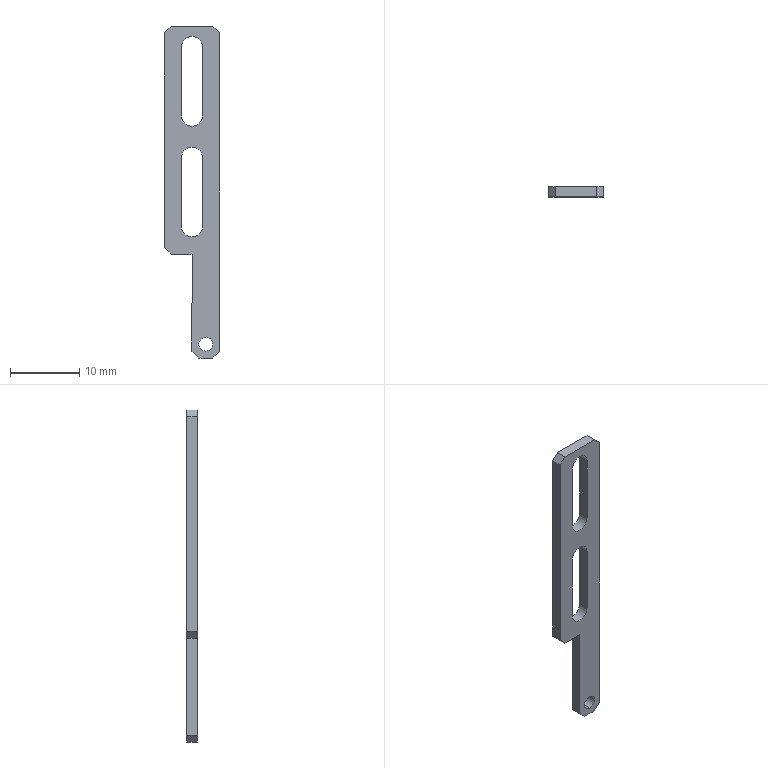Part | SolidWorks | features ICE 3, Chamfer 1, Extrusion 1, HoleWzd 1 | 1 solid | 25 faces | box 8 x 1.5 x 48 mm | volume 366.332 mm3 | plane 17 | cylinder 8 | commonest cylinder face diameters 3 x6 2 x2
STEP:
#1=CARTESIAN_POINT('',(5.5,0.,-3.));
#2=VERTEX_POINT('',#1);
#3=CARTESIAN_POINT('',(4.,0.,-1.5));
#4=VERTEX_POINT('',#3);
#5=CARTESIAN_POINT('',(4.,0.,-3.));
#6=DIRECTION('',(0.,-1.,0.));
#7=DIRECTION('',(0.,0.,-1.));
#8=AXIS2_PLACEMENT_3D('',#5,#6,#7);
#9=CIRCLE('',#8,1.5);
#10=EDGE_CURVE('',#2,#4,#9,.T.);
#11=ORIENTED_EDGE('',*,*,#10,.T.);
#12=CARTESIAN_POINT('',(4.,1.5,-1.5));
#13=VERTEX_POINT('',#12);
#14=CARTESIAN_POINT('',(4.,-8.5,-1.5));
#15=DIRECTION('',(0.,1.,0.));
#16=VECTOR('',#15,1000.);
#17=LINE('',#14,#16);
#18=EDGE_CURVE('',#4,#13,#17,.T.);
#19=ORIENTED_EDGE('',*,*,#18,.T.);
#20=CARTESIAN_POINT('',(5.5,1.5,-3.));
#21=VERTEX_POINT('',#20);
#22=CARTESIAN_POINT('',(4.,1.5,-3.));
#23=DIRECTION('',(0.,1.,0.));
#24=DIRECTION('',(0.,0.,1.));
#25=AXIS2_PLACEMENT_3D('',#22,#23,#24);
#26=CIRCLE('',#25,1.5);
#27=EDGE_CURVE('',#13,#21,#26,.T.);
#28=ORIENTED_EDGE('',*,*,#27,.T.);
#29=CARTESIAN_POINT('',(5.5,-8.5,-3.));
#30=DIRECTION('',(0.,1.,0.));
#31=VECTOR('',#30,1000.);
#32=LINE('',#29,#31);
#33=EDGE_CURVE('',#2,#21,#32,.T.);
#34=ORIENTED_EDGE('',*,*,#33,.F.);
#35=EDGE_LOOP('',(#11,#19,#28,#34));
#36=FACE_OUTER_BOUND('',#35,.T.);
#37=CARTESIAN_POINT('',(4.,-8.5,-3.));
#38=DIRECTION('',(0.,1.,0.));
#39=DIRECTION('',(0.,0.,1.));
#40=AXIS2_PLACEMENT_3D('',#37,#38,#39);
#41=CYLINDRICAL_SURFACE('',#40,1.5);
#42=ADVANCED_FACE('',(#36),#41,.F.);
#43=CARTESIAN_POINT('',(5.5,0.,-19.));
#44=VERTEX_POINT('',#43);
#45=CARTESIAN_POINT('',(4.,0.,-17.5));
#46=VERTEX_POINT('',#45);
#47=CARTESIAN_POINT('',(4.,0.,-19.));
#48=DIRECTION('',(0.,-1.,0.));
#49=DIRECTION('',(0.,0.,-1.));
#50=AXIS2_PLACEMENT_3D('',#47,#48,#49);
#51=CIRCLE('',#50,1.5);
#52=EDGE_CURVE('',#44,#46,#51,.T.);
#53=ORIENTED_EDGE('',*,*,#52,.T.);
#54=CARTESIAN_POINT('',(4.,1.5,-17.5));
#55=VERTEX_POINT('',#54);
#56=CARTESIAN_POINT('',(4.,-8.5,-17.5));
#57=DIRECTION('',(0.,1.,0.));
#58=VECTOR('',#57,1000.);
#59=LINE('',#56,#58);
#60=EDGE_CURVE('',#46,#55,#59,.T.);
#61=ORIENTED_EDGE('',*,*,#60,.T.);
#62=CARTESIAN_POINT('',(5.5,1.5,-19.));
#63=VERTEX_POINT('',#62);
#64=CARTESIAN_POINT('',(4.,1.5,-19.));
#65=DIRECTION('',(0.,1.,0.));
#66=DIRECTION('',(0.,0.,1.));
#67=AXIS2_PLACEMENT_3D('',#64,#65,#66);
#68=CIRCLE('',#67,1.5);
#69=EDGE_CURVE('',#55,#63,#68,.T.);
#70=ORIENTED_EDGE('',*,*,#69,.T.);
#71=CARTESIAN_POINT('',(5.5,-8.5,-19.));
#72=DIRECTION('',(0.,1.,0.));
#73=VECTOR('',#72,1000.);
#74=LINE('',#71,#73);
#75=EDGE_CURVE('',#44,#63,#74,.T.);
#76=ORIENTED_EDGE('',*,*,#75,.F.);
#77=EDGE_LOOP('',(#53,#61,#70,#76));
#78=FACE_OUTER_BOUND('',#77,.T.);
#79=CARTESIAN_POINT('',(4.,-8.5,-19.));
#80=DIRECTION('',(0.,1.,0.));
#81=DIRECTION('',(0.,0.,1.));
#82=AXIS2_PLACEMENT_3D('',#79,#80,#81);
#83=CYLINDRICAL_SURFACE('',#82,1.5);
#84=ADVANCED_FACE('',(#78),#83,.F.);
#85=CARTESIAN_POINT('',(6.,0.,-45.));
#86=VERTEX_POINT('',#85);
#87=CARTESIAN_POINT('',(6.,0.,-47.));
#88=VERTEX_POINT('',#87);
#89=CARTESIAN_POINT('',(6.,0.,-46.));
#90=DIRECTION('',(0.,-1.,0.));
#91=DIRECTION('',(0.,0.,-1.));
#92=AXIS2_PLACEMENT_3D('',#89,#90,#91);
#93=CIRCLE('',#92,1.);
#94=EDGE_CURVE('',#86,#88,#93,.T.);
#95=ORIENTED_EDGE('',*,*,#94,.T.);
#96=CARTESIAN_POINT('',(6.,1.5,-47.));
#97=VERTEX_POINT('',#96);
#98=CARTESIAN_POINT('',(6.,1.5,-47.));
#99=DIRECTION('',(0.,1.,0.));
#100=VECTOR('',#99,1000.);
#101=LINE('',#98,#100);
#102=EDGE_CURVE('',#88,#97,#101,.T.);
#103=ORIENTED_EDGE('',*,*,#102,.T.);
#104=CARTESIAN_POINT('',(6.,1.5,-45.));
#105=VERTEX_POINT('',#104);
#106=CARTESIAN_POINT('',(6.,1.5,-46.));
#107=DIRECTION('',(0.,1.,0.));
#108=DIRECTION('',(0.,0.,1.));
#109=AXIS2_PLACEMENT_3D('',#106,#107,#108);
#110=CIRCLE('',#109,1.);
#111=EDGE_CURVE('',#97,#105,#110,.T.);
#112=ORIENTED_EDGE('',*,*,#111,.T.);
#113=CARTESIAN_POINT('',(6.,1.5,-45.));
#114=DIRECTION('',(0.,1.,0.));
#115=VECTOR('',#114,1000.);
#116=LINE('',#113,#115);
#117=EDGE_CURVE('',#86,#105,#116,.T.);
#118=ORIENTED_EDGE('',*,*,#117,.F.);
#119=EDGE_LOOP('',(#95,#103,#112,#118));
#120=FACE_OUTER_BOUND('',#119,.T.);
#121=CARTESIAN_POINT('',(6.,1.5,-46.));
#122=DIRECTION('',(0.,1.,0.));
#123=DIRECTION('',(0.,0.,1.));
#124=AXIS2_PLACEMENT_3D('',#121,#122,#123);
#125=CYLINDRICAL_SURFACE('',#124,1.);
#126=ADVANCED_FACE('',(#120),#125,.F.);
#127=CARTESIAN_POINT('',(0.,0.,-32.));
#128=VERTEX_POINT('',#127);
#129=CARTESIAN_POINT('',(0.,0.,-1.));
#130=VERTEX_POINT('',#129);
#131=CARTESIAN_POINT('',(0.,0.,0.));
#132=DIRECTION('',(0.,0.,1.));
#133=VECTOR('',#132,1000.);
#134=LINE('',#131,#133);
#135=EDGE_CURVE('',#128,#130,#134,.T.);
#136=ORIENTED_EDGE('',*,*,#135,.T.);
#137=CARTESIAN_POINT('',(0.,1.5,-1.));
#138=VERTEX_POINT('',#137);
#139=CARTESIAN_POINT('',(0.,1.5,-1.));
#140=DIRECTION('',(0.,1.,0.));
#141=VECTOR('',#140,1000.);
#142=LINE('',#139,#141);
#143=EDGE_CURVE('',#130,#138,#142,.T.);
#144=ORIENTED_EDGE('',*,*,#143,.T.);
#145=CARTESIAN_POINT('',(0.,1.5,-32.));
#146=VERTEX_POINT('',#145);
#147=CARTESIAN_POINT('',(0.,1.5,0.));
#148=DIRECTION('',(0.,0.,1.));
#149=VECTOR('',#148,1000.);
#150=LINE('',#147,#149);
#151=EDGE_CURVE('',#146,#138,#150,.T.);
#152=ORIENTED_EDGE('',*,*,#151,.F.);
#153=CARTESIAN_POINT('',(0.,1.5,-32.));
#154=DIRECTION('',(0.,-1.,0.));
#155=VECTOR('',#154,1000.);
#156=LINE('',#153,#155);
#157=EDGE_CURVE('',#146,#128,#156,.T.);
#158=ORIENTED_EDGE('',*,*,#157,.T.);
#159=EDGE_LOOP('',(#136,#144,#152,#158));
#160=FACE_OUTER_BOUND('',#159,.T.);
#161=CARTESIAN_POINT('',(0.,1.5,0.));
#162=DIRECTION('',(1.,0.,0.));
#163=DIRECTION('',(0.,0.,-1.));
#164=AXIS2_PLACEMENT_3D('',#161,#162,#163);
#165=PLANE('',#164);
#166=ADVANCED_FACE('',(#160),#165,.F.);
#167=CARTESIAN_POINT('',(1.,0.,0.));
#168=VERTEX_POINT('',#167);
#169=CARTESIAN_POINT('',(7.,0.,0.));
#170=VERTEX_POINT('',#169);
#171=CARTESIAN_POINT('',(0.,0.,0.));
#172=DIRECTION('',(1.,0.,0.));
#173=VECTOR('',#172,1000.);
#174=LINE('',#171,#173);
#175=EDGE_CURVE('',#168,#170,#174,.T.);
#176=ORIENTED_EDGE('',*,*,#175,.T.);
#177=CARTESIAN_POINT('',(7.,1.5,0.));
#178=VERTEX_POINT('',#177);
#179=CARTESIAN_POINT('',(7.,1.5,0.));
#180=DIRECTION('',(0.,1.,0.));
#181=VECTOR('',#180,1000.);
#182=LINE('',#179,#181);
#183=EDGE_CURVE('',#170,#178,#182,.T.);
#184=ORIENTED_EDGE('',*,*,#183,.T.);
#185=CARTESIAN_POINT('',(1.,1.5,0.));
#186=VERTEX_POINT('',#185);
#187=CARTESIAN_POINT('',(0.,1.5,0.));
#188=DIRECTION('',(1.,0.,0.));
#189=VECTOR('',#188,1000.);
#190=LINE('',#187,#189);
#191=EDGE_CURVE('',#186,#178,#190,.T.);
#192=ORIENTED_EDGE('',*,*,#191,.F.);
#193=CARTESIAN_POINT('',(1.,1.5,0.));
#194=DIRECTION('',(0.,-1.,0.));
#195=VECTOR('',#194,1000.);
#196=LINE('',#193,#195);
#197=EDGE_CURVE('',#186,#168,#196,.T.);
#198=ORIENTED_EDGE('',*,*,#197,.T.);
#199=EDGE_LOOP('',(#176,#184,#192,#198));
#200=FACE_OUTER_BOUND('',#199,.T.);
#201=CARTESIAN_POINT('',(0.,1.5,0.));
#202=DIRECTION('',(0.,0.,-1.));
#203=DIRECTION('',(-1.,0.,0.));
#204=AXIS2_PLACEMENT_3D('',#201,#202,#203);
#205=PLANE('',#204);
#206=ADVANCED_FACE('',(#200),#205,.F.);
#207=CARTESIAN_POINT('',(8.,1.5,-1.));
#208=VERTEX_POINT('',#207);
#209=CARTESIAN_POINT('',(8.,1.5,-47.));
#210=VERTEX_POINT('',#209);
#211=CARTESIAN_POINT('',(8.,1.5,0.));
#212=DIRECTION('',(0.,0.,-1.));
#213=VECTOR('',#212,1000.);
#214=LINE('',#211,#213);
#215=EDGE_CURVE('',#208,#210,#214,.T.);
#216=ORIENTED_EDGE('',*,*,#215,.F.);
#217=CARTESIAN_POINT('',(8.,0.,-1.));
#218=VERTEX_POINT('',#217);
#219=CARTESIAN_POINT('',(8.,1.5,-1.));
#220=DIRECTION('',(0.,-1.,0.));
#221=VECTOR('',#220,1000.);
#222=LINE('',#219,#221);
#223=EDGE_CURVE('',#208,#218,#222,.T.);
#224=ORIENTED_EDGE('',*,*,#223,.T.);
#225=CARTESIAN_POINT('',(8.,0.,-47.));
#226=VERTEX_POINT('',#225);
#227=CARTESIAN_POINT('',(8.,0.,0.));
#228=DIRECTION('',(0.,0.,-1.));
#229=VECTOR('',#228,1000.);
#230=LINE('',#227,#229);
#231=EDGE_CURVE('',#218,#226,#230,.T.);
#232=ORIENTED_EDGE('',*,*,#231,.T.);
#233=CARTESIAN_POINT('',(8.,1.5,-47.));
#234=DIRECTION('',(0.,1.,0.));
#235=VECTOR('',#234,1000.);
#236=LINE('',#233,#235);
#237=EDGE_CURVE('',#226,#210,#236,.T.);
#238=ORIENTED_EDGE('',*,*,#237,.T.);
#239=EDGE_LOOP('',(#216,#224,#232,#238));
#240=FACE_OUTER_BOUND('',#239,.T.);
#241=CARTESIAN_POINT('',(8.,1.5,0.));
#242=DIRECTION('',(-1.,0.,0.));
#243=DIRECTION('',(0.,0.,1.));
#244=AXIS2_PLACEMENT_3D('',#241,#242,#243);
#245=PLANE('',#244);
#246=ADVANCED_FACE('',(#240),#245,.F.);
#247=CARTESIAN_POINT('',(7.,0.,-48.));
#248=VERTEX_POINT('',#247);
#249=CARTESIAN_POINT('',(5.,0.,-48.));
#250=VERTEX_POINT('',#249);
#251=CARTESIAN_POINT('',(0.,0.,-48.));
#252=DIRECTION('',(-1.,0.,0.));
#253=VECTOR('',#252,1000.);
#254=LINE('',#251,#253);
#255=EDGE_CURVE('',#248,#250,#254,.T.);
#256=ORIENTED_EDGE('',*,*,#255,.T.);
#257=CARTESIAN_POINT('',(5.,1.5,-48.));
#258=VERTEX_POINT('',#257);
#259=CARTESIAN_POINT('',(5.,1.5,-48.));
#260=DIRECTION('',(0.,1.,0.));
#261=VECTOR('',#260,1000.);
#262=LINE('',#259,#261);
#263=EDGE_CURVE('',#250,#258,#262,.T.);
#264=ORIENTED_EDGE('',*,*,#263,.T.);
#265=CARTESIAN_POINT('',(7.,1.5,-48.));
#266=VERTEX_POINT('',#265);
#267=CARTESIAN_POINT('',(0.,1.5,-48.));
#268=DIRECTION('',(-1.,0.,0.));
#269=VECTOR('',#268,1000.);
#270=LINE('',#267,#269);
#271=EDGE_CURVE('',#266,#258,#270,.T.);
#272=ORIENTED_EDGE('',*,*,#271,.F.);
#273=CARTESIAN_POINT('',(7.,1.5,-48.));
#274=DIRECTION('',(0.,-1.,0.));
#275=VECTOR('',#274,1000.);
#276=LINE('',#273,#275);
#277=EDGE_CURVE('',#266,#248,#276,.T.);
#278=ORIENTED_EDGE('',*,*,#277,.T.);
#279=EDGE_LOOP('',(#256,#264,#272,#278));
#280=FACE_OUTER_BOUND('',#279,.T.);
#281=CARTESIAN_POINT('',(0.,1.5,-48.));
#282=DIRECTION('',(0.,0.,1.));
#283=DIRECTION('',(1.,0.,0.));
#284=AXIS2_PLACEMENT_3D('',#281,#282,#283);
#285=PLANE('',#284);
#286=ADVANCED_FACE('',(#280),#285,.F.);
#287=CARTESIAN_POINT('',(5.5,1.5,-13.));
#288=VERTEX_POINT('',#287);
#289=CARTESIAN_POINT('',(5.5,1.5,-3.));
#290=DIRECTION('',(0.,0.,-1.));
#291=VECTOR('',#290,1000.);
#292=LINE('',#289,#291);
#293=EDGE_CURVE('',#21,#288,#292,.T.);
#294=ORIENTED_EDGE('',*,*,#293,.F.);
#295=ORIENTED_EDGE('',*,*,#27,.F.);
#296=CARTESIAN_POINT('',(2.5,1.5,-3.));
#297=VERTEX_POINT('',#296);
#298=CARTESIAN_POINT('',(4.,1.5,-3.));
#299=DIRECTION('',(0.,1.,0.));
#300=DIRECTION('',(0.,0.,1.));
#301=AXIS2_PLACEMENT_3D('',#298,#299,#300);
#302=CIRCLE('',#301,1.5);
#303=EDGE_CURVE('',#297,#13,#302,.T.);
#304=ORIENTED_EDGE('',*,*,#303,.F.);
#305=CARTESIAN_POINT('',(2.5,1.5,-13.));
#306=VERTEX_POINT('',#305);
#307=CARTESIAN_POINT('',(2.5,1.5,-3.));
#308=DIRECTION('',(0.,0.,1.));
#309=VECTOR('',#308,1000.);
#310=LINE('',#307,#309);
#311=EDGE_CURVE('',#306,#297,#310,.T.);
#312=ORIENTED_EDGE('',*,*,#311,.F.);
#313=CARTESIAN_POINT('',(4.,1.5,-13.));
#314=DIRECTION('',(0.,1.,0.));
#315=DIRECTION('',(0.,0.,1.));
#316=AXIS2_PLACEMENT_3D('',#313,#314,#315);
#317=CIRCLE('',#316,1.5);
#318=EDGE_CURVE('',#288,#306,#317,.T.);
#319=ORIENTED_EDGE('',*,*,#318,.F.);
#320=EDGE_LOOP('',(#294,#295,#304,#312,#319));
#321=FACE_BOUND('',#320,.T.);
#322=CARTESIAN_POINT('',(2.5,1.5,-29.));
#323=VERTEX_POINT('',#322);
#324=CARTESIAN_POINT('',(2.5,1.5,-19.));
#325=VERTEX_POINT('',#324);
#326=CARTESIAN_POINT('',(2.5,1.5,-29.));
#327=DIRECTION('',(0.,0.,1.));
#328=VECTOR('',#327,1000.);
#329=LINE('',#326,#328);
#330=EDGE_CURVE('',#323,#325,#329,.T.);
#331=ORIENTED_EDGE('',*,*,#330,.F.);
#332=CARTESIAN_POINT('',(5.5,1.5,-29.));
#333=VERTEX_POINT('',#332);
#334=CARTESIAN_POINT('',(4.,1.5,-29.));
#335=DIRECTION('',(0.,1.,0.));
#336=DIRECTION('',(0.,0.,1.));
#337=AXIS2_PLACEMENT_3D('',#334,#335,#336);
#338=CIRCLE('',#337,1.5);
#339=EDGE_CURVE('',#333,#323,#338,.T.);
#340=ORIENTED_EDGE('',*,*,#339,.F.);
#341=CARTESIAN_POINT('',(5.5,1.5,-29.));
#342=DIRECTION('',(0.,0.,-1.));
#343=VECTOR('',#342,1000.);
#344=LINE('',#341,#343);
#345=EDGE_CURVE('',#63,#333,#344,.T.);
#346=ORIENTED_EDGE('',*,*,#345,.F.);
#347=ORIENTED_EDGE('',*,*,#69,.F.);
#348=CARTESIAN_POINT('',(4.,1.5,-19.));
#349=DIRECTION('',(0.,1.,0.));
#350=DIRECTION('',(0.,0.,1.));
#351=AXIS2_PLACEMENT_3D('',#348,#349,#350);
#352=CIRCLE('',#351,1.5);
#353=EDGE_CURVE('',#325,#55,#352,.T.);
#354=ORIENTED_EDGE('',*,*,#353,.F.);
#355=EDGE_LOOP('',(#331,#340,#346,#347,#354));
#356=FACE_BOUND('',#355,.T.);
#357=CARTESIAN_POINT('',(6.,1.5,-46.));
#358=DIRECTION('',(0.,1.,0.));
#359=DIRECTION('',(0.,0.,1.));
#360=AXIS2_PLACEMENT_3D('',#357,#358,#359);
#361=CIRCLE('',#360,1.);
#362=EDGE_CURVE('',#105,#97,#361,.T.);
#363=ORIENTED_EDGE('',*,*,#362,.F.);
#364=ORIENTED_EDGE('',*,*,#111,.F.);
#365=EDGE_LOOP('',(#363,#364));
#366=FACE_BOUND('',#365,.T.);
#367=ORIENTED_EDGE('',*,*,#191,.T.);
#368=CARTESIAN_POINT('',(8.,1.5,-1.));
#369=DIRECTION('',(0.7071,0.,-0.7071));
#370=VECTOR('',#369,1000.);
#371=LINE('',#368,#370);
#372=EDGE_CURVE('',#178,#208,#371,.T.);
#373=ORIENTED_EDGE('',*,*,#372,.T.);
#374=ORIENTED_EDGE('',*,*,#215,.T.);
#375=CARTESIAN_POINT('',(7.,1.5,-48.));
#376=DIRECTION('',(-0.7071,0.,-0.7071));
#377=VECTOR('',#376,1000.);
#378=LINE('',#375,#377);
#379=EDGE_CURVE('',#210,#266,#378,.T.);
#380=ORIENTED_EDGE('',*,*,#379,.T.);
#381=ORIENTED_EDGE('',*,*,#271,.T.);
#382=CARTESIAN_POINT('',(4.,1.5,-47.));
#383=VERTEX_POINT('',#382);
#384=CARTESIAN_POINT('',(5.,1.5,-48.));
#385=DIRECTION('',(-0.7071,0.,0.7071));
#386=VECTOR('',#385,1000.);
#387=LINE('',#384,#386);
#388=EDGE_CURVE('',#258,#383,#387,.T.);
#389=ORIENTED_EDGE('',*,*,#388,.T.);
#390=CARTESIAN_POINT('',(4.,1.5,-33.));
#391=VERTEX_POINT('',#390);
#392=CARTESIAN_POINT('',(4.,1.5,-48.));
#393=DIRECTION('',(0.,0.,-1.));
#394=VECTOR('',#393,1000.);
#395=LINE('',#392,#394);
#396=EDGE_CURVE('',#391,#383,#395,.T.);
#397=ORIENTED_EDGE('',*,*,#396,.F.);
#398=CARTESIAN_POINT('',(1.,1.5,-33.));
#399=VERTEX_POINT('',#398);
#400=CARTESIAN_POINT('',(0.,1.5,-33.));
#401=DIRECTION('',(1.,0.,0.));
#402=VECTOR('',#401,1000.);
#403=LINE('',#400,#402);
#404=EDGE_CURVE('',#399,#391,#403,.T.);
#405=ORIENTED_EDGE('',*,*,#404,.F.);
#406=CARTESIAN_POINT('',(1.,1.5,-33.));
#407=DIRECTION('',(-0.7071,0.,0.7071));
#408=VECTOR('',#407,1000.);
#409=LINE('',#406,#408);
#410=EDGE_CURVE('',#399,#146,#409,.T.);
#411=ORIENTED_EDGE('',*,*,#410,.T.);
#412=ORIENTED_EDGE('',*,*,#151,.T.);
#413=CARTESIAN_POINT('',(1.,1.5,0.));
#414=DIRECTION('',(0.7071,0.,0.7071));
#415=VECTOR('',#414,1000.);
#416=LINE('',#413,#415);
#417=EDGE_CURVE('',#138,#186,#416,.T.);
#418=ORIENTED_EDGE('',*,*,#417,.T.);
#419=EDGE_LOOP('',(#367,#373,#374,#380,#381,#389,#397,#405,#411,#412,#418));
#420=FACE_OUTER_BOUND('',#419,.T.);
#421=CARTESIAN_POINT('',(0.,1.5,0.));
#422=DIRECTION('',(0.,-1.,0.));
#423=DIRECTION('',(0.,0.,-1.));
#424=AXIS2_PLACEMENT_3D('',#421,#422,#423);
#425=PLANE('',#424);
#426=ADVANCED_FACE('',(#321,#356,#366,#420),#425,.F.);
#427=ORIENTED_EDGE('',*,*,#10,.F.);
#428=CARTESIAN_POINT('',(5.5,0.,-13.));
#429=VERTEX_POINT('',#428);
#430=CARTESIAN_POINT('',(5.5,0.,0.));
#431=DIRECTION('',(0.,0.,1.));
#432=VECTOR('',#431,1000.);
#433=LINE('',#430,#432);
#434=EDGE_CURVE('',#429,#2,#433,.T.);
#435=ORIENTED_EDGE('',*,*,#434,.F.);
#436=CARTESIAN_POINT('',(2.5,0.,-13.));
#437=VERTEX_POINT('',#436);
#438=CARTESIAN_POINT('',(4.,0.,-13.));
#439=DIRECTION('',(0.,-1.,0.));
#440=DIRECTION('',(0.,0.,-1.));
#441=AXIS2_PLACEMENT_3D('',#438,#439,#440);
#442=CIRCLE('',#441,1.5);
#443=EDGE_CURVE('',#437,#429,#442,.T.);
#444=ORIENTED_EDGE('',*,*,#443,.F.);
#445=CARTESIAN_POINT('',(2.5,0.,-3.));
#446=VERTEX_POINT('',#445);
#447=CARTESIAN_POINT('',(2.5,0.,0.));
#448=DIRECTION('',(0.,0.,-1.));
#449=VECTOR('',#448,1000.);
#450=LINE('',#447,#449);
#451=EDGE_CURVE('',#446,#437,#450,.T.);
#452=ORIENTED_EDGE('',*,*,#451,.F.);
#453=CARTESIAN_POINT('',(4.,0.,-3.));
#454=DIRECTION('',(0.,-1.,0.));
#455=DIRECTION('',(0.,0.,-1.));
#456=AXIS2_PLACEMENT_3D('',#453,#454,#455);
#457=CIRCLE('',#456,1.5);
#458=EDGE_CURVE('',#4,#446,#457,.T.);
#459=ORIENTED_EDGE('',*,*,#458,.F.);
#460=EDGE_LOOP('',(#427,#435,#444,#452,#459));
#461=FACE_BOUND('',#460,.T.);
#462=CARTESIAN_POINT('',(2.5,0.,-29.));
#463=VERTEX_POINT('',#462);
#464=CARTESIAN_POINT('',(5.5,0.,-29.));
#465=VERTEX_POINT('',#464);
#466=CARTESIAN_POINT('',(4.,0.,-29.));
#467=DIRECTION('',(0.,-1.,0.));
#468=DIRECTION('',(0.,0.,-1.));
#469=AXIS2_PLACEMENT_3D('',#466,#467,#468);
#470=CIRCLE('',#469,1.5);
#471=EDGE_CURVE('',#463,#465,#470,.T.);
#472=ORIENTED_EDGE('',*,*,#471,.F.);
#473=CARTESIAN_POINT('',(2.5,0.,-19.));
#474=VERTEX_POINT('',#473);
#475=CARTESIAN_POINT('',(2.5,0.,0.));
#476=DIRECTION('',(0.,0.,-1.));
#477=VECTOR('',#476,1000.);
#478=LINE('',#475,#477);
#479=EDGE_CURVE('',#474,#463,#478,.T.);
#480=ORIENTED_EDGE('',*,*,#479,.F.);
#481=CARTESIAN_POINT('',(4.,0.,-19.));
#482=DIRECTION('',(0.,-1.,0.));
#483=DIRECTION('',(0.,0.,-1.));
#484=AXIS2_PLACEMENT_3D('',#481,#482,#483);
#485=CIRCLE('',#484,1.5);
#486=EDGE_CURVE('',#46,#474,#485,.T.);
#487=ORIENTED_EDGE('',*,*,#486,.F.);
#488=ORIENTED_EDGE('',*,*,#52,.F.);
#489=CARTESIAN_POINT('',(5.5,0.,0.));
#490=DIRECTION('',(0.,0.,1.));
#491=VECTOR('',#490,1000.);
#492=LINE('',#489,#491);
#493=EDGE_CURVE('',#465,#44,#492,.T.);
#494=ORIENTED_EDGE('',*,*,#493,.F.);
#495=EDGE_LOOP('',(#472,#480,#487,#488,#494));
#496=FACE_BOUND('',#495,.T.);
#497=ORIENTED_EDGE('',*,*,#231,.F.);
#498=CARTESIAN_POINT('',(3.5,0.,3.5));
#499=DIRECTION('',(-0.7071,0.,0.7071));
#500=VECTOR('',#499,1000.);
#501=LINE('',#498,#500);
#502=EDGE_CURVE('',#218,#170,#501,.T.);
#503=ORIENTED_EDGE('',*,*,#502,.T.);
#504=ORIENTED_EDGE('',*,*,#175,.F.);
#505=CARTESIAN_POINT('',(0.5,0.,-0.5));
#506=DIRECTION('',(-0.7071,0.,-0.7071));
#507=VECTOR('',#506,1000.);
#508=LINE('',#505,#507);
#509=EDGE_CURVE('',#168,#130,#508,.T.);
#510=ORIENTED_EDGE('',*,*,#509,.T.);
#511=ORIENTED_EDGE('',*,*,#135,.F.);
#512=CARTESIAN_POINT('',(1.,0.,-33.));
#513=VERTEX_POINT('',#512);
#514=CARTESIAN_POINT('',(-16.,0.,-16.));
#515=DIRECTION('',(0.7071,0.,-0.7071));
#516=VECTOR('',#515,1000.);
#517=LINE('',#514,#516);
#518=EDGE_CURVE('',#128,#513,#517,.T.);
#519=ORIENTED_EDGE('',*,*,#518,.T.);
#520=CARTESIAN_POINT('',(4.,0.,-33.));
#521=VERTEX_POINT('',#520);
#522=CARTESIAN_POINT('',(0.,0.,-33.));
#523=DIRECTION('',(-1.,0.,0.));
#524=VECTOR('',#523,1000.);
#525=LINE('',#522,#524);
#526=EDGE_CURVE('',#521,#513,#525,.T.);
#527=ORIENTED_EDGE('',*,*,#526,.F.);
#528=CARTESIAN_POINT('',(4.,0.,-47.));
#529=VERTEX_POINT('',#528);
#530=CARTESIAN_POINT('',(4.,0.,0.));
#531=DIRECTION('',(0.,0.,1.));
#532=VECTOR('',#531,1000.);
#533=LINE('',#530,#532);
#534=EDGE_CURVE('',#529,#521,#533,.T.);
#535=ORIENTED_EDGE('',*,*,#534,.F.);
#536=CARTESIAN_POINT('',(-21.5,0.,-21.5));
#537=DIRECTION('',(0.7071,0.,-0.7071));
#538=VECTOR('',#537,1000.);
#539=LINE('',#536,#538);
#540=EDGE_CURVE('',#529,#250,#539,.T.);
#541=ORIENTED_EDGE('',*,*,#540,.T.);
#542=ORIENTED_EDGE('',*,*,#255,.F.);
#543=CARTESIAN_POINT('',(27.5,0.,-27.5));
#544=DIRECTION('',(0.7071,0.,0.7071));
#545=VECTOR('',#544,1000.);
#546=LINE('',#543,#545);
#547=EDGE_CURVE('',#248,#226,#546,.T.);
#548=ORIENTED_EDGE('',*,*,#547,.T.);
#549=EDGE_LOOP('',(#497,#503,#504,#510,#511,#519,#527,#535,#541,#542,#548));
#550=FACE_OUTER_BOUND('',#549,.T.);
#551=ORIENTED_EDGE('',*,*,#94,.F.);
#552=CARTESIAN_POINT('',(6.,0.,-46.));
#553=DIRECTION('',(0.,-1.,0.));
#554=DIRECTION('',(0.,0.,-1.));
#555=AXIS2_PLACEMENT_3D('',#552,#553,#554);
#556=CIRCLE('',#555,1.);
#557=EDGE_CURVE('',#88,#86,#556,.T.);
#558=ORIENTED_EDGE('',*,*,#557,.F.);
#559=EDGE_LOOP('',(#551,#558));
#560=FACE_BOUND('',#559,.T.);
#561=CARTESIAN_POINT('',(0.,0.,0.));
#562=DIRECTION('',(0.,-1.,0.));
#563=DIRECTION('',(0.,0.,-1.));
#564=AXIS2_PLACEMENT_3D('',#561,#562,#563);
#565=PLANE('',#564);
#566=ADVANCED_FACE('',(#461,#496,#550,#560),#565,.T.);
#567=ORIENTED_EDGE('',*,*,#102,.F.);
#568=ORIENTED_EDGE('',*,*,#557,.T.);
#569=ORIENTED_EDGE('',*,*,#117,.T.);
#570=ORIENTED_EDGE('',*,*,#362,.T.);
#571=EDGE_LOOP('',(#567,#568,#569,#570));
#572=FACE_OUTER_BOUND('',#571,.T.);
#573=CARTESIAN_POINT('',(6.,1.5,-46.));
#574=DIRECTION('',(0.,1.,0.));
#575=DIRECTION('',(0.,0.,1.));
#576=AXIS2_PLACEMENT_3D('',#573,#574,#575);
#577=CYLINDRICAL_SURFACE('',#576,1.);
#578=ADVANCED_FACE('',(#572),#577,.F.);
#579=ORIENTED_EDGE('',*,*,#396,.T.);
#580=CARTESIAN_POINT('',(4.,-8.5,-47.));
#581=DIRECTION('',(0.,-1.,0.));
#582=VECTOR('',#581,1000.);
#583=LINE('',#580,#582);
#584=EDGE_CURVE('',#383,#529,#583,.T.);
#585=ORIENTED_EDGE('',*,*,#584,.T.);
#586=ORIENTED_EDGE('',*,*,#534,.T.);
#587=CARTESIAN_POINT('',(4.,-8.5,-33.));
#588=DIRECTION('',(0.,1.,0.));
#589=VECTOR('',#588,1000.);
#590=LINE('',#587,#589);
#591=EDGE_CURVE('',#521,#391,#590,.T.);
#592=ORIENTED_EDGE('',*,*,#591,.T.);
#593=EDGE_LOOP('',(#579,#585,#586,#592));
#594=FACE_OUTER_BOUND('',#593,.T.);
#595=CARTESIAN_POINT('',(4.,-8.5,-48.));
#596=DIRECTION('',(1.,0.,0.));
#597=DIRECTION('',(0.,0.,-1.));
#598=AXIS2_PLACEMENT_3D('',#595,#596,#597);
#599=PLANE('',#598);
#600=ADVANCED_FACE('',(#594),#599,.F.);
#601=ORIENTED_EDGE('',*,*,#526,.T.);
#602=CARTESIAN_POINT('',(1.,-8.5,-33.));
#603=DIRECTION('',(0.,1.,0.));
#604=VECTOR('',#603,1000.);
#605=LINE('',#602,#604);
#606=EDGE_CURVE('',#513,#399,#605,.T.);
#607=ORIENTED_EDGE('',*,*,#606,.T.);
#608=ORIENTED_EDGE('',*,*,#404,.T.);
#609=ORIENTED_EDGE('',*,*,#591,.F.);
#610=EDGE_LOOP('',(#601,#607,#608,#609));
#611=FACE_OUTER_BOUND('',#610,.T.);
#612=CARTESIAN_POINT('',(0.,-8.5,-33.));
#613=DIRECTION('',(0.,0.,1.));
#614=DIRECTION('',(1.,0.,0.));
#615=AXIS2_PLACEMENT_3D('',#612,#613,#614);
#616=PLANE('',#615);
#617=ADVANCED_FACE('',(#611),#616,.F.);
#618=ORIENTED_EDGE('',*,*,#372,.F.);
#619=ORIENTED_EDGE('',*,*,#183,.F.);
#620=ORIENTED_EDGE('',*,*,#502,.F.);
#621=ORIENTED_EDGE('',*,*,#223,.F.);
#622=EDGE_LOOP('',(#618,#619,#620,#621));
#623=FACE_OUTER_BOUND('',#622,.T.);
#624=CARTESIAN_POINT('',(8.,1.5,-1.));
#625=DIRECTION('',(-0.7071,0.,-0.7071));
#626=DIRECTION('',(0.,-1.,0.));
#627=AXIS2_PLACEMENT_3D('',#624,#625,#626);
#628=PLANE('',#627);
#629=ADVANCED_FACE('',(#623),#628,.F.);
#630=ORIENTED_EDGE('',*,*,#417,.F.);
#631=ORIENTED_EDGE('',*,*,#143,.F.);
#632=ORIENTED_EDGE('',*,*,#509,.F.);
#633=ORIENTED_EDGE('',*,*,#197,.F.);
#634=EDGE_LOOP('',(#630,#631,#632,#633));
#635=FACE_OUTER_BOUND('',#634,.T.);
#636=CARTESIAN_POINT('',(1.,1.5,0.));
#637=DIRECTION('',(0.7071,0.,-0.7071));
#638=DIRECTION('',(0.,-1.,0.));
#639=AXIS2_PLACEMENT_3D('',#636,#637,#638);
#640=PLANE('',#639);
#641=ADVANCED_FACE('',(#635),#640,.F.);
#642=ORIENTED_EDGE('',*,*,#518,.F.);
#643=ORIENTED_EDGE('',*,*,#157,.F.);
#644=ORIENTED_EDGE('',*,*,#410,.F.);
#645=ORIENTED_EDGE('',*,*,#606,.F.);
#646=EDGE_LOOP('',(#642,#643,#644,#645));
#647=FACE_OUTER_BOUND('',#646,.T.);
#648=CARTESIAN_POINT('',(1.,-8.5,-33.));
#649=DIRECTION('',(0.7071,0.,0.7071));
#650=DIRECTION('',(0.,1.,0.));
#651=AXIS2_PLACEMENT_3D('',#648,#649,#650);
#652=PLANE('',#651);
#653=ADVANCED_FACE('',(#647),#652,.F.);
#654=ORIENTED_EDGE('',*,*,#540,.F.);
#655=ORIENTED_EDGE('',*,*,#584,.F.);
#656=ORIENTED_EDGE('',*,*,#388,.F.);
#657=ORIENTED_EDGE('',*,*,#263,.F.);
#658=EDGE_LOOP('',(#654,#655,#656,#657));
#659=FACE_OUTER_BOUND('',#658,.T.);
#660=CARTESIAN_POINT('',(5.,1.5,-48.));
#661=DIRECTION('',(0.7071,0.,0.7071));
#662=DIRECTION('',(0.,1.,0.));
#663=AXIS2_PLACEMENT_3D('',#660,#661,#662);
#664=PLANE('',#663);
#665=ADVANCED_FACE('',(#659),#664,.F.);
#666=ORIENTED_EDGE('',*,*,#379,.F.);
#667=ORIENTED_EDGE('',*,*,#237,.F.);
#668=ORIENTED_EDGE('',*,*,#547,.F.);
#669=ORIENTED_EDGE('',*,*,#277,.F.);
#670=EDGE_LOOP('',(#666,#667,#668,#669));
#671=FACE_OUTER_BOUND('',#670,.T.);
#672=CARTESIAN_POINT('',(7.,1.5,-48.));
#673=DIRECTION('',(-0.7071,0.,0.7071));
#674=DIRECTION('',(0.,-1.,0.));
#675=AXIS2_PLACEMENT_3D('',#672,#673,#674);
#676=PLANE('',#675);
#677=ADVANCED_FACE('',(#671),#676,.F.);
#678=ORIENTED_EDGE('',*,*,#493,.T.);
#679=ORIENTED_EDGE('',*,*,#75,.T.);
#680=ORIENTED_EDGE('',*,*,#345,.T.);
#681=CARTESIAN_POINT('',(5.5,-8.5,-29.));
#682=DIRECTION('',(0.,1.,0.));
#683=VECTOR('',#682,1000.);
#684=LINE('',#681,#683);
#685=EDGE_CURVE('',#465,#333,#684,.T.);
#686=ORIENTED_EDGE('',*,*,#685,.F.);
#687=EDGE_LOOP('',(#678,#679,#680,#686));
#688=FACE_OUTER_BOUND('',#687,.T.);
#689=CARTESIAN_POINT('',(5.5,-8.5,-29.));
#690=DIRECTION('',(1.,0.,0.));
#691=DIRECTION('',(0.,0.,-1.));
#692=AXIS2_PLACEMENT_3D('',#689,#690,#691);
#693=PLANE('',#692);
#694=ADVANCED_FACE('',(#688),#693,.F.);
#695=ORIENTED_EDGE('',*,*,#479,.T.);
#696=CARTESIAN_POINT('',(2.5,-8.5,-29.));
#697=DIRECTION('',(0.,1.,0.));
#698=VECTOR('',#697,1000.);
#699=LINE('',#696,#698);
#700=EDGE_CURVE('',#463,#323,#699,.T.);
#701=ORIENTED_EDGE('',*,*,#700,.T.);
#702=ORIENTED_EDGE('',*,*,#330,.T.);
#703=CARTESIAN_POINT('',(2.5,-8.5,-19.));
#704=DIRECTION('',(0.,1.,0.));
#705=VECTOR('',#704,1000.);
#706=LINE('',#703,#705);
#707=EDGE_CURVE('',#474,#325,#706,.T.);
#708=ORIENTED_EDGE('',*,*,#707,.F.);
#709=EDGE_LOOP('',(#695,#701,#702,#708));
#710=FACE_OUTER_BOUND('',#709,.T.);
#711=CARTESIAN_POINT('',(2.5,-8.5,-29.));
#712=DIRECTION('',(-1.,0.,0.));
#713=DIRECTION('',(0.,0.,1.));
#714=AXIS2_PLACEMENT_3D('',#711,#712,#713);
#715=PLANE('',#714);
#716=ADVANCED_FACE('',(#710),#715,.F.);
#717=ORIENTED_EDGE('',*,*,#471,.T.);
#718=ORIENTED_EDGE('',*,*,#685,.T.);
#719=ORIENTED_EDGE('',*,*,#339,.T.);
#720=ORIENTED_EDGE('',*,*,#700,.F.);
#721=EDGE_LOOP('',(#717,#718,#719,#720));
#722=FACE_OUTER_BOUND('',#721,.T.);
#723=CARTESIAN_POINT('',(4.,-8.5,-29.));
#724=DIRECTION('',(0.,1.,0.));
#725=DIRECTION('',(0.,0.,1.));
#726=AXIS2_PLACEMENT_3D('',#723,#724,#725);
#727=CYLINDRICAL_SURFACE('',#726,1.5);
#728=ADVANCED_FACE('',(#722),#727,.F.);
#729=ORIENTED_EDGE('',*,*,#60,.F.);
#730=ORIENTED_EDGE('',*,*,#486,.T.);
#731=ORIENTED_EDGE('',*,*,#707,.T.);
#732=ORIENTED_EDGE('',*,*,#353,.T.);
#733=EDGE_LOOP('',(#729,#730,#731,#732));
#734=FACE_OUTER_BOUND('',#733,.T.);
#735=CARTESIAN_POINT('',(4.,-8.5,-19.));
#736=DIRECTION('',(0.,1.,0.));
#737=DIRECTION('',(0.,0.,1.));
#738=AXIS2_PLACEMENT_3D('',#735,#736,#737);
#739=CYLINDRICAL_SURFACE('',#738,1.5);
#740=ADVANCED_FACE('',(#734),#739,.F.);
#741=ORIENTED_EDGE('',*,*,#451,.T.);
#742=CARTESIAN_POINT('',(2.5,-8.5,-13.));
#743=DIRECTION('',(0.,1.,0.));
#744=VECTOR('',#743,1000.);
#745=LINE('',#742,#744);
#746=EDGE_CURVE('',#437,#306,#745,.T.);
#747=ORIENTED_EDGE('',*,*,#746,.T.);
#748=ORIENTED_EDGE('',*,*,#311,.T.);
#749=CARTESIAN_POINT('',(2.5,-8.5,-3.));
#750=DIRECTION('',(0.,1.,0.));
#751=VECTOR('',#750,1000.);
#752=LINE('',#749,#751);
#753=EDGE_CURVE('',#446,#297,#752,.T.);
#754=ORIENTED_EDGE('',*,*,#753,.F.);
#755=EDGE_LOOP('',(#741,#747,#748,#754));
#756=FACE_OUTER_BOUND('',#755,.T.);
#757=CARTESIAN_POINT('',(2.5,-8.5,-3.));
#758=DIRECTION('',(-1.,0.,0.));
#759=DIRECTION('',(0.,0.,1.));
#760=AXIS2_PLACEMENT_3D('',#757,#758,#759);
#761=PLANE('',#760);
#762=ADVANCED_FACE('',(#756),#761,.F.);
#763=ORIENTED_EDGE('',*,*,#434,.T.);
#764=ORIENTED_EDGE('',*,*,#33,.T.);
#765=ORIENTED_EDGE('',*,*,#293,.T.);
#766=CARTESIAN_POINT('',(5.5,-8.5,-13.));
#767=DIRECTION('',(0.,1.,0.));
#768=VECTOR('',#767,1000.);
#769=LINE('',#766,#768);
#770=EDGE_CURVE('',#429,#288,#769,.T.);
#771=ORIENTED_EDGE('',*,*,#770,.F.);
#772=EDGE_LOOP('',(#763,#764,#765,#771));
#773=FACE_OUTER_BOUND('',#772,.T.);
#774=CARTESIAN_POINT('',(5.5,-8.5,-3.));
#775=DIRECTION('',(1.,0.,0.));
#776=DIRECTION('',(0.,0.,-1.));
#777=AXIS2_PLACEMENT_3D('',#774,#775,#776);
#778=PLANE('',#777);
#779=ADVANCED_FACE('',(#773),#778,.F.);
#780=ORIENTED_EDGE('',*,*,#18,.F.);
#781=ORIENTED_EDGE('',*,*,#458,.T.);
#782=ORIENTED_EDGE('',*,*,#753,.T.);
#783=ORIENTED_EDGE('',*,*,#303,.T.);
#784=EDGE_LOOP('',(#780,#781,#782,#783));
#785=FACE_OUTER_BOUND('',#784,.T.);
#786=CARTESIAN_POINT('',(4.,-8.5,-3.));
#787=DIRECTION('',(0.,1.,0.));
#788=DIRECTION('',(0.,0.,1.));
#789=AXIS2_PLACEMENT_3D('',#786,#787,#788);
#790=CYLINDRICAL_SURFACE('',#789,1.5);
#791=ADVANCED_FACE('',(#785),#790,.F.);
#792=ORIENTED_EDGE('',*,*,#443,.T.);
#793=ORIENTED_EDGE('',*,*,#770,.T.);
#794=ORIENTED_EDGE('',*,*,#318,.T.);
#795=ORIENTED_EDGE('',*,*,#746,.F.);
#796=EDGE_LOOP('',(#792,#793,#794,#795));
#797=FACE_OUTER_BOUND('',#796,.T.);
#798=CARTESIAN_POINT('',(4.,-8.5,-13.));
#799=DIRECTION('',(0.,1.,0.));
#800=DIRECTION('',(0.,0.,1.));
#801=AXIS2_PLACEMENT_3D('',#798,#799,#800);
#802=CYLINDRICAL_SURFACE('',#801,1.5);
#803=ADVANCED_FACE('',(#797),#802,.F.);
#804=CLOSED_SHELL('',(#42,#84,#126,#166,#206,#246,#286,#426,#566,#578,#600,#617,#629,#641,#653,#665,#677,#694,#716,#728,#740,#762,#779,#791,#803));
#805=MANIFOLD_SOLID_BREP('',#804);
#806=CARTESIAN_POINT('',(0.,0.,0.));
#807=DIRECTION('',(0.,0.,1.));
#808=DIRECTION('',(1.,0.,0.));
#809=AXIS2_PLACEMENT_3D('',#806,#807,#808);
#810=(LENGTH_UNIT()NAMED_UNIT(*)SI_UNIT(.MILLI.,.METRE.));
#811=UNCERTAINTY_MEASURE_WITH_UNIT(LENGTH_MEASURE(0.00001),#810,'','');
#812=(NAMED_UNIT(*)PLANE_ANGLE_UNIT()SI_UNIT($,.RADIAN.));
#813=(NAMED_UNIT(*)SI_UNIT($,.STERADIAN.)SOLID_ANGLE_UNIT());
#814=(GEOMETRIC_REPRESENTATION_CONTEXT(3)GLOBAL_UNCERTAINTY_ASSIGNED_CONTEXT((#811))GLOBAL_UNIT_ASSIGNED_CONTEXT((#810,#812,#813))REPRESENTATION_CONTEXT('',''));
#815=ADVANCED_BREP_SHAPE_REPRESENTATION('',(#805,#809),#814);